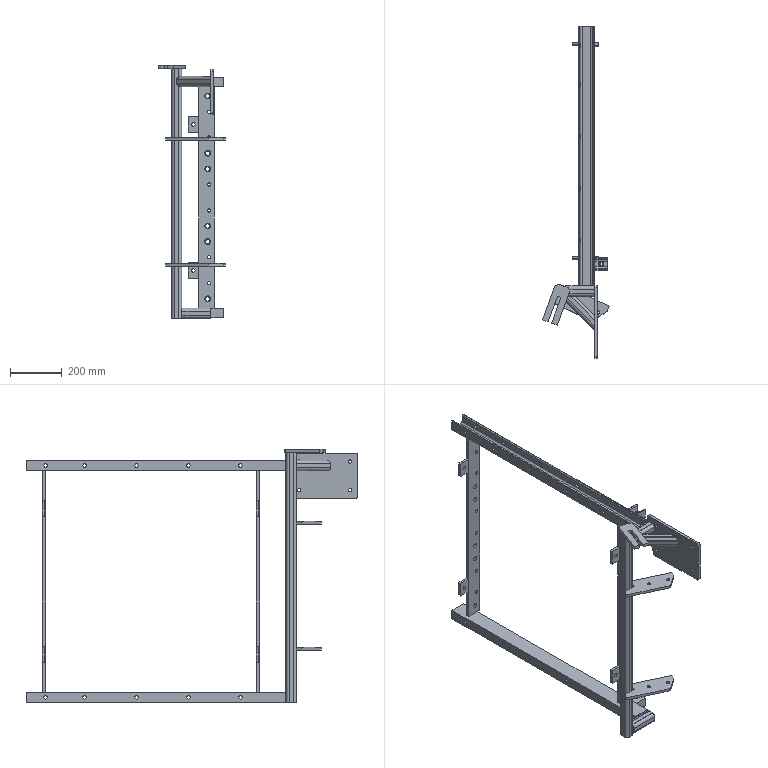Part | SolidWorks | features LayoutProfileFeature 1 | 20 solids | 408 faces | box 257.243 x 1277 x 974 mm | volume 4686993 mm3 | cylinder 196 | plane 180 | cone 32 | commonest cylinder face diameters 13 x92 17 x24 22 x24 16 x16 24 x16 14 x5